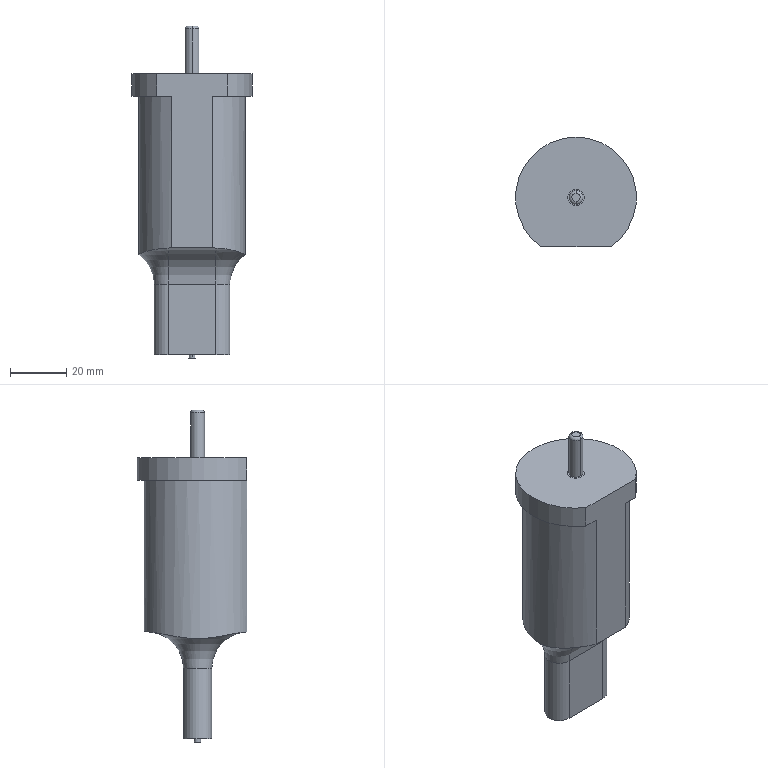Part | STEP file | 1_id290_x_t | 1 solid | 28 faces | box 43 x 39 x 118.2 mm | volume 84183 mm3 | cylinder 14 | plane 10 | torus 4 | commonest cylinder face diameters 2.26 x2 5 x2 6 x2 10.07 x2 26 x2 38 x2
STEP:
#1=CARTESIAN_POINT('',(3411.,-73.993,30.458));
#2=VERTEX_POINT('',#1);
#3=CARTESIAN_POINT('',(3412.101,-74.5,30.489));
#4=VERTEX_POINT('',#3);
#5=CARTESIAN_POINT('',(3411.,-73.993,30.458));
#6=CARTESIAN_POINT('',(3411.361,-74.173,30.473));
#7=CARTESIAN_POINT('',(3411.729,-74.343,30.483));
#8=CARTESIAN_POINT('',(3412.101,-74.5,30.489));
#9=B_SPLINE_CURVE_WITH_KNOTS('',3,(#5,#6,#7,#8),.UNSPECIFIED.,.F.,.F.,(4,4),(0.,1.),.UNSPECIFIED.);
#10=EDGE_CURVE('',#2,#4,#9,.T.);
#11=ORIENTED_EDGE('',*,*,#10,.T.);
#12=CARTESIAN_POINT('',(3412.101,-74.5,84.5));
#13=VERTEX_POINT('',#12);
#14=CARTESIAN_POINT('',(3412.101,-74.5,38.5));
#15=DIRECTION('',(0.,0.,1.));
#16=VECTOR('',#15,1.);
#17=LINE('',#14,#16);
#18=EDGE_CURVE('',#4,#13,#17,.T.);
#19=ORIENTED_EDGE('',*,*,#18,.T.);
#20=CARTESIAN_POINT('',(3419.5,-38.,84.5));
#21=VERTEX_POINT('',#20);
#22=CARTESIAN_POINT('',(3419.5,-57.,84.5));
#23=DIRECTION('',(0.,0.,1.));
#24=DIRECTION('',(0.,1.,0.));
#25=AXIS2_PLACEMENT_3D('',#22,#23,#24);
#26=CIRCLE('',#25,19.);
#27=EDGE_CURVE('',#21,#13,#26,.T.);
#28=ORIENTED_EDGE('',*,*,#27,.F.);
#29=CARTESIAN_POINT('',(3419.5,-38.,30.5));
#30=VERTEX_POINT('',#29);
#31=CARTESIAN_POINT('',(3419.5,-38.,38.5));
#32=DIRECTION('',(0.,0.,1.));
#33=VECTOR('',#32,1.);
#34=LINE('',#31,#33);
#35=EDGE_CURVE('',#30,#21,#34,.T.);
#36=ORIENTED_EDGE('',*,*,#35,.F.);
#37=CARTESIAN_POINT('',(3413.522,-38.965,30.5));
#38=VERTEX_POINT('',#37);
#39=CARTESIAN_POINT('',(3419.5,-57.,30.5));
#40=DIRECTION('',(0.,0.,1.));
#41=DIRECTION('',(0.,1.,0.));
#42=AXIS2_PLACEMENT_3D('',#39,#40,#41);
#43=CIRCLE('',#42,19.);
#44=EDGE_CURVE('',#30,#38,#43,.T.);
#45=ORIENTED_EDGE('',*,*,#44,.T.);
#46=CARTESIAN_POINT('',(3411.,-40.007,30.458));
#47=VERTEX_POINT('',#46);
#48=CARTESIAN_POINT('',(3413.522,-38.965,30.5));
#49=CARTESIAN_POINT('',(3412.658,-39.251,30.5));
#50=CARTESIAN_POINT('',(3411.813,-39.601,30.491));
#51=CARTESIAN_POINT('',(3411.,-40.007,30.458));
#52=B_SPLINE_CURVE_WITH_KNOTS('',3,(#48,#49,#50,#51),.UNSPECIFIED.,.F.,.F.,(4,4),(0.,1.),.UNSPECIFIED.);
#53=EDGE_CURVE('',#38,#47,#52,.T.);
#54=ORIENTED_EDGE('',*,*,#53,.T.);
#55=CARTESIAN_POINT('',(3411.,-40.007,30.458));
#56=CARTESIAN_POINT('',(3407.815,-41.601,30.33));
#57=CARTESIAN_POINT('',(3405.165,-44.053,29.874));
#58=CARTESIAN_POINT('',(3401.509,-49.97,28.735));
#59=CARTESIAN_POINT('',(3400.502,-53.482,28.095));
#60=CARTESIAN_POINT('',(3400.498,-60.5,28.093));
#61=CARTESIAN_POINT('',(3401.497,-64.005,28.73));
#62=CARTESIAN_POINT('',(3405.163,-69.948,29.874));
#63=CARTESIAN_POINT('',(3407.814,-72.399,30.33));
#64=CARTESIAN_POINT('',(3411.,-73.993,30.458));
#65=B_SPLINE_CURVE_WITH_KNOTS('',3,(#55,#56,#57,#58,#59,#60,#61,#62,#63,#64),.UNSPECIFIED.,.F.,.F.,(4,2,2,2,4),(0.,0.25,0.5,0.75,1.),.UNSPECIFIED.);
#66=EDGE_CURVE('',#47,#2,#65,.T.);
#67=ORIENTED_EDGE('',*,*,#66,.T.);
#68=EDGE_LOOP('',(#11,#19,#28,#36,#45,#54,#67));
#69=FACE_OUTER_BOUND('',#68,.T.);
#70=CARTESIAN_POINT('',(3419.5,-57.,38.5));
#71=DIRECTION('',(0.,0.,-1.));
#72=DIRECTION('',(0.,-1.,0.));
#73=AXIS2_PLACEMENT_3D('',#70,#71,#72);
#74=CYLINDRICAL_SURFACE('',#73,19.);
#75=ADVANCED_FACE('',(#69),#74,.T.);
#76=CARTESIAN_POINT('',(3419.5,-35.5,84.5));
#77=VERTEX_POINT('',#76);
#78=CARTESIAN_POINT('',(3407.01,-74.5,84.5));
#79=VERTEX_POINT('',#78);
#80=CARTESIAN_POINT('',(3419.5,-57.,84.5));
#81=DIRECTION('',(0.,0.,1.));
#82=DIRECTION('',(0.,1.,0.));
#83=AXIS2_PLACEMENT_3D('',#80,#81,#82);
#84=CIRCLE('',#83,21.5);
#85=EDGE_CURVE('',#77,#79,#84,.T.);
#86=ORIENTED_EDGE('',*,*,#85,.T.);
#87=CARTESIAN_POINT('',(3407.01,-74.5,92.5));
#88=VERTEX_POINT('',#87);
#89=CARTESIAN_POINT('',(3407.01,-74.5,88.5));
#90=DIRECTION('',(0.,0.,-1.));
#91=VECTOR('',#90,1.);
#92=LINE('',#89,#91);
#93=EDGE_CURVE('',#88,#79,#92,.T.);
#94=ORIENTED_EDGE('',*,*,#93,.F.);
#95=CARTESIAN_POINT('',(3419.5,-35.5,92.5));
#96=VERTEX_POINT('',#95);
#97=CARTESIAN_POINT('',(3419.5,-57.,92.5));
#98=DIRECTION('',(0.,0.,1.));
#99=DIRECTION('',(0.,1.,0.));
#100=AXIS2_PLACEMENT_3D('',#97,#98,#99);
#101=CIRCLE('',#100,21.5);
#102=EDGE_CURVE('',#96,#88,#101,.T.);
#103=ORIENTED_EDGE('',*,*,#102,.F.);
#104=CARTESIAN_POINT('',(3419.5,-35.5,88.5));
#105=DIRECTION('',(0.,0.,1.));
#106=VECTOR('',#105,1.);
#107=LINE('',#104,#106);
#108=EDGE_CURVE('',#77,#96,#107,.T.);
#109=ORIENTED_EDGE('',*,*,#108,.F.);
#110=EDGE_LOOP('',(#86,#94,#103,#109));
#111=FACE_OUTER_BOUND('',#110,.T.);
#112=CARTESIAN_POINT('',(3419.5,-57.,88.5));
#113=DIRECTION('',(0.,0.,-1.));
#114=DIRECTION('',(0.,-1.,0.));
#115=AXIS2_PLACEMENT_3D('',#112,#113,#114);
#116=CYLINDRICAL_SURFACE('',#115,21.5);
#117=ADVANCED_FACE('',(#111),#116,.T.);
#118=CARTESIAN_POINT('',(3431.99,-74.5,92.5));
#119=VERTEX_POINT('',#118);
#120=CARTESIAN_POINT('',(3419.5,-57.,92.5));
#121=DIRECTION('',(0.,0.,1.));
#122=DIRECTION('',(0.,1.,0.));
#123=AXIS2_PLACEMENT_3D('',#120,#121,#122);
#124=CIRCLE('',#123,21.5);
#125=EDGE_CURVE('',#119,#96,#124,.T.);
#126=ORIENTED_EDGE('',*,*,#125,.F.);
#127=CARTESIAN_POINT('',(3431.99,-74.5,84.5));
#128=VERTEX_POINT('',#127);
#129=CARTESIAN_POINT('',(3431.99,-74.5,88.5));
#130=DIRECTION('',(0.,0.,-1.));
#131=VECTOR('',#130,1.);
#132=LINE('',#129,#131);
#133=EDGE_CURVE('',#119,#128,#132,.T.);
#134=ORIENTED_EDGE('',*,*,#133,.T.);
#135=CARTESIAN_POINT('',(3419.5,-57.,84.5));
#136=DIRECTION('',(0.,0.,1.));
#137=DIRECTION('',(0.,1.,0.));
#138=AXIS2_PLACEMENT_3D('',#135,#136,#137);
#139=CIRCLE('',#138,21.5);
#140=EDGE_CURVE('',#128,#77,#139,.T.);
#141=ORIENTED_EDGE('',*,*,#140,.T.);
#142=ORIENTED_EDGE('',*,*,#108,.T.);
#143=EDGE_LOOP('',(#126,#134,#141,#142));
#144=FACE_OUTER_BOUND('',#143,.T.);
#145=CARTESIAN_POINT('',(3419.5,-57.,88.5));
#146=DIRECTION('',(0.,0.,-1.));
#147=DIRECTION('',(0.,-1.,0.));
#148=AXIS2_PLACEMENT_3D('',#145,#146,#147);
#149=CYLINDRICAL_SURFACE('',#148,21.5);
#150=ADVANCED_FACE('',(#144),#149,.T.);
#151=ORIENTED_EDGE('',*,*,#140,.F.);
#152=CARTESIAN_POINT('',(3426.899,-74.5,84.5));
#153=VERTEX_POINT('',#152);
#154=CARTESIAN_POINT('',(3419.5,-74.5,84.5));
#155=DIRECTION('',(-1.,0.,0.));
#156=VECTOR('',#155,1.);
#157=LINE('',#154,#156);
#158=EDGE_CURVE('',#128,#153,#157,.T.);
#159=ORIENTED_EDGE('',*,*,#158,.T.);
#160=CARTESIAN_POINT('',(3419.5,-57.,84.5));
#161=DIRECTION('',(0.,0.,1.));
#162=DIRECTION('',(0.,1.,0.));
#163=AXIS2_PLACEMENT_3D('',#160,#161,#162);
#164=CIRCLE('',#163,19.);
#165=EDGE_CURVE('',#153,#21,#164,.T.);
#166=ORIENTED_EDGE('',*,*,#165,.T.);
#167=ORIENTED_EDGE('',*,*,#27,.T.);
#168=CARTESIAN_POINT('',(3419.5,-74.5,84.5));
#169=DIRECTION('',(-1.,0.,0.));
#170=VECTOR('',#169,1.);
#171=LINE('',#168,#170);
#172=EDGE_CURVE('',#13,#79,#171,.T.);
#173=ORIENTED_EDGE('',*,*,#172,.T.);
#174=ORIENTED_EDGE('',*,*,#85,.F.);
#175=EDGE_LOOP('',(#151,#159,#166,#167,#173,#174));
#176=FACE_OUTER_BOUND('',#175,.T.);
#177=CARTESIAN_POINT('',(3419.5,-36.75,84.5));
#178=DIRECTION('',(0.,0.,-1.));
#179=DIRECTION('',(0.,1.,0.));
#180=AXIS2_PLACEMENT_3D('',#177,#178,#179);
#181=PLANE('',#180);
#182=ADVANCED_FACE('',(#176),#181,.T.);
#183=CARTESIAN_POINT('',(3426.899,-74.5,30.489));
#184=VERTEX_POINT('',#183);
#185=CARTESIAN_POINT('',(3457.5,-74.5,30.489));
#186=DIRECTION('',(1.,0.,0.));
#187=VECTOR('',#186,1.);
#188=LINE('',#185,#187);
#189=EDGE_CURVE('',#4,#184,#188,.T.);
#190=ORIENTED_EDGE('',*,*,#189,.F.);
#191=ORIENTED_EDGE('',*,*,#10,.F.);
#192=CARTESIAN_POINT('',(3411.,-62.035,17.5));
#193=VERTEX_POINT('',#192);
#194=CARTESIAN_POINT('',(3411.,-75.035,17.5));
#195=DIRECTION('',(-1.,0.,0.));
#196=DIRECTION('',(0.,-1.,0.));
#197=AXIS2_PLACEMENT_3D('',#194,#195,#196);
#198=CIRCLE('',#197,13.);
#199=EDGE_CURVE('',#2,#193,#198,.T.);
#200=ORIENTED_EDGE('',*,*,#199,.T.);
#201=CARTESIAN_POINT('',(3428.,-62.035,17.5));
#202=VERTEX_POINT('',#201);
#203=CARTESIAN_POINT('',(3457.5,-62.035,17.5));
#204=DIRECTION('',(-1.,0.,0.));
#205=VECTOR('',#204,1.);
#206=LINE('',#203,#205);
#207=EDGE_CURVE('',#202,#193,#206,.T.);
#208=ORIENTED_EDGE('',*,*,#207,.F.);
#209=CARTESIAN_POINT('',(3428.,-73.993,30.458));
#210=VERTEX_POINT('',#209);
#211=CARTESIAN_POINT('',(3428.,-75.035,17.5));
#212=DIRECTION('',(1.,0.,0.));
#213=DIRECTION('',(0.,-1.,0.));
#214=AXIS2_PLACEMENT_3D('',#211,#212,#213);
#215=CIRCLE('',#214,13.);
#216=EDGE_CURVE('',#202,#210,#215,.T.);
#217=ORIENTED_EDGE('',*,*,#216,.T.);
#218=CARTESIAN_POINT('',(3426.899,-74.5,30.489));
#219=CARTESIAN_POINT('',(3427.272,-74.343,30.483));
#220=CARTESIAN_POINT('',(3427.639,-74.173,30.473));
#221=CARTESIAN_POINT('',(3428.,-73.993,30.458));
#222=B_SPLINE_CURVE_WITH_KNOTS('',3,(#218,#219,#220,#221),.UNSPECIFIED.,.F.,.F.,(4,4),(0.,1.),.UNSPECIFIED.);
#223=EDGE_CURVE('',#184,#210,#222,.T.);
#224=ORIENTED_EDGE('',*,*,#223,.F.);
#225=EDGE_LOOP('',(#190,#191,#200,#208,#217,#224));
#226=FACE_OUTER_BOUND('',#225,.T.);
#227=CARTESIAN_POINT('',(3457.5,-75.035,17.5));
#228=DIRECTION('',(1.,0.,0.));
#229=DIRECTION('',(0.,-1.,0.));
#230=AXIS2_PLACEMENT_3D('',#227,#228,#229);
#231=CYLINDRICAL_SURFACE('',#230,13.);
#232=ADVANCED_FACE('',(#226),#231,.F.);
#233=ORIENTED_EDGE('',*,*,#165,.F.);
#234=CARTESIAN_POINT('',(3426.899,-74.5,38.5));
#235=DIRECTION('',(0.,0.,-1.));
#236=VECTOR('',#235,1.);
#237=LINE('',#234,#236);
#238=EDGE_CURVE('',#153,#184,#237,.T.);
#239=ORIENTED_EDGE('',*,*,#238,.T.);
#240=ORIENTED_EDGE('',*,*,#223,.T.);
#241=CARTESIAN_POINT('',(3428.,-40.007,30.458));
#242=VERTEX_POINT('',#241);
#243=CARTESIAN_POINT('',(3428.,-73.993,30.458));
#244=CARTESIAN_POINT('',(3431.185,-72.399,30.33));
#245=CARTESIAN_POINT('',(3433.835,-69.947,29.874));
#246=CARTESIAN_POINT('',(3437.491,-64.03,28.735));
#247=CARTESIAN_POINT('',(3438.498,-60.518,28.095));
#248=CARTESIAN_POINT('',(3438.502,-53.5,28.093));
#249=CARTESIAN_POINT('',(3437.503,-49.995,28.73));
#250=CARTESIAN_POINT('',(3433.837,-44.052,29.874));
#251=CARTESIAN_POINT('',(3431.186,-41.601,30.33));
#252=CARTESIAN_POINT('',(3428.,-40.007,30.458));
#253=B_SPLINE_CURVE_WITH_KNOTS('',3,(#243,#244,#245,#246,#247,#248,#249,#250,#251,#252),.UNSPECIFIED.,.F.,.F.,(4,2,2,2,4),(0.,0.25,0.5,0.75,1.),.UNSPECIFIED.);
#254=EDGE_CURVE('',#210,#242,#253,.T.);
#255=ORIENTED_EDGE('',*,*,#254,.T.);
#256=CARTESIAN_POINT('',(3425.478,-38.965,30.5));
#257=VERTEX_POINT('',#256);
#258=CARTESIAN_POINT('',(3428.,-40.007,30.458));
#259=CARTESIAN_POINT('',(3427.187,-39.601,30.491));
#260=CARTESIAN_POINT('',(3426.342,-39.251,30.5));
#261=CARTESIAN_POINT('',(3425.478,-38.965,30.5));
#262=B_SPLINE_CURVE_WITH_KNOTS('',3,(#258,#259,#260,#261),.UNSPECIFIED.,.F.,.F.,(4,4),(0.,1.),.UNSPECIFIED.);
#263=EDGE_CURVE('',#242,#257,#262,.T.);
#264=ORIENTED_EDGE('',*,*,#263,.T.);
#265=CARTESIAN_POINT('',(3419.5,-57.,30.5));
#266=DIRECTION('',(0.,0.,1.));
#267=DIRECTION('',(0.,1.,0.));
#268=AXIS2_PLACEMENT_3D('',#265,#266,#267);
#269=CIRCLE('',#268,19.);
#270=EDGE_CURVE('',#257,#30,#269,.T.);
#271=ORIENTED_EDGE('',*,*,#270,.T.);
#272=ORIENTED_EDGE('',*,*,#35,.T.);
#273=EDGE_LOOP('',(#233,#239,#240,#255,#264,#271,#272));
#274=FACE_OUTER_BOUND('',#273,.T.);
#275=CARTESIAN_POINT('',(3419.5,-57.,38.5));
#276=DIRECTION('',(0.,0.,-1.));
#277=DIRECTION('',(0.,-1.,0.));
#278=AXIS2_PLACEMENT_3D('',#275,#276,#277);
#279=CYLINDRICAL_SURFACE('',#278,19.);
#280=ADVANCED_FACE('',(#274),#279,.T.);
#281=CARTESIAN_POINT('',(3419.5,-54.,92.5));
#282=VERTEX_POINT('',#281);
#283=CARTESIAN_POINT('',(3419.5,-60.,92.5));
#284=VERTEX_POINT('',#283);
#285=CARTESIAN_POINT('',(3419.5,-57.,92.5));
#286=DIRECTION('',(0.,0.,-1.));
#287=DIRECTION('',(0.,-1.,0.));
#288=AXIS2_PLACEMENT_3D('',#285,#286,#287);
#289=CIRCLE('',#288,3.);
#290=EDGE_CURVE('',#282,#284,#289,.T.);
#291=ORIENTED_EDGE('',*,*,#290,.T.);
#292=CARTESIAN_POINT('',(3419.5,-57.,92.5));
#293=DIRECTION('',(0.,0.,-1.));
#294=DIRECTION('',(0.,-1.,0.));
#295=AXIS2_PLACEMENT_3D('',#292,#293,#294);
#296=CIRCLE('',#295,3.);
#297=EDGE_CURVE('',#284,#282,#296,.T.);
#298=ORIENTED_EDGE('',*,*,#297,.T.);
#299=EDGE_LOOP('',(#291,#298));
#300=FACE_BOUND('',#299,.T.);
#301=ORIENTED_EDGE('',*,*,#102,.T.);
#302=CARTESIAN_POINT('',(3419.5,-74.5,92.5));
#303=DIRECTION('',(-1.,0.,0.));
#304=VECTOR('',#303,1.);
#305=LINE('',#302,#304);
#306=EDGE_CURVE('',#119,#88,#305,.T.);
#307=ORIENTED_EDGE('',*,*,#306,.F.);
#308=ORIENTED_EDGE('',*,*,#125,.T.);
#309=EDGE_LOOP('',(#301,#307,#308));
#310=FACE_BOUND('',#309,.T.);
#311=CARTESIAN_POINT('',(3419.5,-46.25,92.5));
#312=DIRECTION('',(0.,0.,1.));
#313=DIRECTION('',(0.,-1.,0.));
#314=AXIS2_PLACEMENT_3D('',#311,#312,#313);
#315=PLANE('',#314);
#316=ADVANCED_FACE('',(#300,#310),#315,.T.);
#317=CARTESIAN_POINT('',(3419.5,-58.13,-7.5));
#318=VERTEX_POINT('',#317);
#319=CARTESIAN_POINT('',(3419.5,-58.13,-8.7));
#320=VERTEX_POINT('',#319);
#321=CARTESIAN_POINT('',(3419.5,-58.13,-7.5));
#322=DIRECTION('',(0.,0.,-1.));
#323=VECTOR('',#322,1.);
#324=LINE('',#321,#323);
#325=EDGE_CURVE('',#318,#320,#324,.T.);
#326=ORIENTED_EDGE('',*,*,#325,.F.);
#327=CARTESIAN_POINT('',(3419.5,-55.87,-7.5));
#328=VERTEX_POINT('',#327);
#329=CARTESIAN_POINT('',(3419.5,-57.,-7.5));
#330=DIRECTION('',(0.,0.,1.));
#331=DIRECTION('',(0.,-1.,0.));
#332=AXIS2_PLACEMENT_3D('',#329,#330,#331);
#333=CIRCLE('',#332,1.13);
#334=EDGE_CURVE('',#328,#318,#333,.T.);
#335=ORIENTED_EDGE('',*,*,#334,.F.);
#336=CARTESIAN_POINT('',(3419.5,-55.87,-8.7));
#337=VERTEX_POINT('',#336);
#338=CARTESIAN_POINT('',(3419.5,-55.87,-7.5));
#339=DIRECTION('',(0.,0.,1.));
#340=VECTOR('',#339,1.);
#341=LINE('',#338,#340);
#342=EDGE_CURVE('',#337,#328,#341,.T.);
#343=ORIENTED_EDGE('',*,*,#342,.F.);
#344=CARTESIAN_POINT('',(3419.5,-57.,-8.7));
#345=DIRECTION('',(0.,0.,1.));
#346=DIRECTION('',(0.,-1.,0.));
#347=AXIS2_PLACEMENT_3D('',#344,#345,#346);
#348=CIRCLE('',#347,1.13);
#349=EDGE_CURVE('',#337,#320,#348,.T.);
#350=ORIENTED_EDGE('',*,*,#349,.T.);
#351=EDGE_LOOP('',(#326,#335,#343,#350));
#352=FACE_OUTER_BOUND('',#351,.T.);
#353=CARTESIAN_POINT('',(3419.5,-57.,-7.5));
#354=DIRECTION('',(0.,0.,1.));
#355=DIRECTION('',(0.,1.,0.));
#356=AXIS2_PLACEMENT_3D('',#353,#354,#355);
#357=CYLINDRICAL_SURFACE('',#356,1.13);
#358=ADVANCED_FACE('',(#352),#357,.T.);
#359=CARTESIAN_POINT('',(3419.5,-59.5,108.5));
#360=VERTEX_POINT('',#359);
#361=CARTESIAN_POINT('',(3419.5,-59.5,92.6));
#362=VERTEX_POINT('',#361);
#363=CARTESIAN_POINT('',(3419.5,-59.5,100.55));
#364=DIRECTION('',(0.,0.,-1.));
#365=VECTOR('',#364,1.);
#366=LINE('',#363,#365);
#367=EDGE_CURVE('',#360,#362,#366,.T.);
#368=ORIENTED_EDGE('',*,*,#367,.F.);
#369=CARTESIAN_POINT('',(3419.5,-54.5,108.5));
#370=VERTEX_POINT('',#369);
#371=CARTESIAN_POINT('',(3419.5,-57.,108.5));
#372=DIRECTION('',(0.,0.,-1.));
#373=DIRECTION('',(0.,-1.,0.));
#374=AXIS2_PLACEMENT_3D('',#371,#372,#373);
#375=CIRCLE('',#374,2.5);
#376=EDGE_CURVE('',#360,#370,#375,.T.);
#377=ORIENTED_EDGE('',*,*,#376,.T.);
#378=CARTESIAN_POINT('',(3419.5,-54.5,92.6));
#379=VERTEX_POINT('',#378);
#380=CARTESIAN_POINT('',(3419.5,-54.5,100.55));
#381=DIRECTION('',(0.,0.,1.));
#382=VECTOR('',#381,1.);
#383=LINE('',#380,#382);
#384=EDGE_CURVE('',#379,#370,#383,.T.);
#385=ORIENTED_EDGE('',*,*,#384,.F.);
#386=CARTESIAN_POINT('',(3419.5,-57.,92.6));
#387=DIRECTION('',(0.,0.,-1.));
#388=DIRECTION('',(0.,-1.,0.));
#389=AXIS2_PLACEMENT_3D('',#386,#387,#388);
#390=CIRCLE('',#389,2.5);
#391=EDGE_CURVE('',#362,#379,#390,.T.);
#392=ORIENTED_EDGE('',*,*,#391,.F.);
#393=EDGE_LOOP('',(#368,#377,#385,#392));
#394=FACE_OUTER_BOUND('',#393,.T.);
#395=CARTESIAN_POINT('',(3419.5,-57.,100.55));
#396=DIRECTION('',(0.,0.,1.));
#397=DIRECTION('',(0.,1.,0.));
#398=AXIS2_PLACEMENT_3D('',#395,#396,#397);
#399=CYLINDRICAL_SURFACE('',#398,2.5);
#400=ADVANCED_FACE('',(#394),#399,.T.);
#401=CARTESIAN_POINT('',(3419.5,-55.5,109.5));
#402=VERTEX_POINT('',#401);
#403=CARTESIAN_POINT('',(3419.5,-55.5,108.5));
#404=DIRECTION('',(-1.,0.,0.));
#405=DIRECTION('',(0.,1.,0.));
#406=AXIS2_PLACEMENT_3D('',#403,#404,#405);
#407=CIRCLE('',#406,1.);
#408=EDGE_CURVE('',#402,#370,#407,.T.);
#409=ORIENTED_EDGE('',*,*,#408,.F.);
#410=CARTESIAN_POINT('',(3419.5,-58.5,109.5));
#411=VERTEX_POINT('',#410);
#412=CARTESIAN_POINT('',(3419.5,-57.,109.5));
#413=DIRECTION('',(0.,0.,-1.));
#414=DIRECTION('',(0.,-1.,0.));
#415=AXIS2_PLACEMENT_3D('',#412,#413,#414);
#416=CIRCLE('',#415,1.5);
#417=EDGE_CURVE('',#402,#411,#416,.T.);
#418=ORIENTED_EDGE('',*,*,#417,.T.);
#419=CARTESIAN_POINT('',(3419.5,-58.5,108.5));
#420=DIRECTION('',(-1.,0.,0.));
#421=DIRECTION('',(0.,-1.,0.));
#422=AXIS2_PLACEMENT_3D('',#419,#420,#421);
#423=CIRCLE('',#422,1.);
#424=EDGE_CURVE('',#360,#411,#423,.T.);
#425=ORIENTED_EDGE('',*,*,#424,.F.);
#426=CARTESIAN_POINT('',(3419.5,-57.,108.5));
#427=DIRECTION('',(0.,0.,-1.));
#428=DIRECTION('',(0.,-1.,0.));
#429=AXIS2_PLACEMENT_3D('',#426,#427,#428);
#430=CIRCLE('',#429,2.5);
#431=EDGE_CURVE('',#370,#360,#430,.T.);
#432=ORIENTED_EDGE('',*,*,#431,.F.);
#433=EDGE_LOOP('',(#409,#418,#425,#432));
#434=FACE_OUTER_BOUND('',#433,.T.);
#435=CARTESIAN_POINT('',(3419.5,-57.,108.5));
#436=DIRECTION('',(0.,0.,-1.));
#437=DIRECTION('',(0.,-1.,0.));
#438=AXIS2_PLACEMENT_3D('',#435,#436,#437);
#439=TOROIDAL_SURFACE('',#438,1.5,1.);
#440=ADVANCED_FACE('',(#434),#439,.T.);
#441=CARTESIAN_POINT('',(3419.5,-60.,92.6));
#442=VERTEX_POINT('',#441);
#443=CARTESIAN_POINT('',(3419.5,-60.,92.55));
#444=DIRECTION('',(0.,0.,-1.));
#445=VECTOR('',#444,1.);
#446=LINE('',#443,#445);
#447=EDGE_CURVE('',#442,#284,#446,.T.);
#448=ORIENTED_EDGE('',*,*,#447,.F.);
#449=CARTESIAN_POINT('',(3419.5,-54.,92.6));
#450=VERTEX_POINT('',#449);
#451=CARTESIAN_POINT('',(3419.5,-57.,92.6));
#452=DIRECTION('',(0.,0.,-1.));
#453=DIRECTION('',(0.,-1.,0.));
#454=AXIS2_PLACEMENT_3D('',#451,#452,#453);
#455=CIRCLE('',#454,3.);
#456=EDGE_CURVE('',#442,#450,#455,.T.);
#457=ORIENTED_EDGE('',*,*,#456,.T.);
#458=CARTESIAN_POINT('',(3419.5,-54.,92.55));
#459=DIRECTION('',(0.,0.,1.));
#460=VECTOR('',#459,1.);
#461=LINE('',#458,#460);
#462=EDGE_CURVE('',#282,#450,#461,.T.);
#463=ORIENTED_EDGE('',*,*,#462,.F.);
#464=ORIENTED_EDGE('',*,*,#297,.F.);
#465=EDGE_LOOP('',(#448,#457,#463,#464));
#466=FACE_OUTER_BOUND('',#465,.T.);
#467=CARTESIAN_POINT('',(3419.5,-57.,87.05));
#468=DIRECTION('',(0.,0.,1.));
#469=DIRECTION('',(0.,1.,0.));
#470=AXIS2_PLACEMENT_3D('',#467,#468,#469);
#471=CYLINDRICAL_SURFACE('',#470,3.);
#472=ADVANCED_FACE('',(#466),#471,.T.);
#473=ORIENTED_EDGE('',*,*,#447,.T.);
#474=ORIENTED_EDGE('',*,*,#290,.F.);
#475=ORIENTED_EDGE('',*,*,#462,.T.);
#476=CARTESIAN_POINT('',(3419.5,-57.,92.6));
#477=DIRECTION('',(0.,0.,-1.));
#478=DIRECTION('',(0.,-1.,0.));
#479=AXIS2_PLACEMENT_3D('',#476,#477,#478);
#480=CIRCLE('',#479,3.);
#481=EDGE_CURVE('',#450,#442,#480,.T.);
#482=ORIENTED_EDGE('',*,*,#481,.T.);
#483=EDGE_LOOP('',(#473,#474,#475,#482));
#484=FACE_OUTER_BOUND('',#483,.T.);
#485=CARTESIAN_POINT('',(3419.5,-57.,87.05));
#486=DIRECTION('',(0.,0.,1.));
#487=DIRECTION('',(0.,1.,0.));
#488=AXIS2_PLACEMENT_3D('',#485,#486,#487);
#489=CYLINDRICAL_SURFACE('',#488,3.);
#490=ADVANCED_FACE('',(#484),#489,.T.);
#491=CARTESIAN_POINT('',(3419.5,-57.,109.5));
#492=DIRECTION('',(0.,0.,-1.));
#493=DIRECTION('',(0.,-1.,0.));
#494=AXIS2_PLACEMENT_3D('',#491,#492,#493);
#495=CIRCLE('',#494,1.5);
#496=EDGE_CURVE('',#411,#402,#495,.T.);
#497=ORIENTED_EDGE('',*,*,#496,.F.);
#498=ORIENTED_EDGE('',*,*,#417,.F.);
#499=EDGE_LOOP('',(#497,#498));
#500=FACE_OUTER_BOUND('',#499,.T.);
#501=CARTESIAN_POINT('',(3419.5,-57.75,109.5));
#502=DIRECTION('',(0.,0.,1.));
#503=DIRECTION('',(0.,-1.,0.));
#504=AXIS2_PLACEMENT_3D('',#501,#502,#503);
#505=PLANE('',#504);
#506=ADVANCED_FACE('',(#500),#505,.T.);
#507=ORIENTED_EDGE('',*,*,#408,.T.);
#508=ORIENTED_EDGE('',*,*,#376,.F.);
#509=ORIENTED_EDGE('',*,*,#424,.T.);
#510=ORIENTED_EDGE('',*,*,#496,.T.);
#511=EDGE_LOOP('',(#507,#508,#509,#510));
#512=FACE_OUTER_BOUND('',#511,.T.);
#513=CARTESIAN_POINT('',(3419.5,-57.,108.5));
#514=DIRECTION('',(0.,0.,-1.));
#515=DIRECTION('',(0.,-1.,0.));
#516=AXIS2_PLACEMENT_3D('',#513,#514,#515);
#517=TOROIDAL_SURFACE('',#516,1.5,1.);
#518=ADVANCED_FACE('',(#512),#517,.T.);
#519=ORIENTED_EDGE('',*,*,#367,.T.);
#520=CARTESIAN_POINT('',(3419.5,-57.,92.6));
#521=DIRECTION('',(0.,0.,-1.));
#522=DIRECTION('',(0.,-1.,0.));
#523=AXIS2_PLACEMENT_3D('',#520,#521,#522);
#524=CIRCLE('',#523,2.5);
#525=EDGE_CURVE('',#379,#362,#524,.T.);
#526=ORIENTED_EDGE('',*,*,#525,.F.);
#527=ORIENTED_EDGE('',*,*,#384,.T.);
#528=ORIENTED_EDGE('',*,*,#431,.T.);
#529=EDGE_LOOP('',(#519,#526,#527,#528));
#530=FACE_OUTER_BOUND('',#529,.T.);
#531=CARTESIAN_POINT('',(3419.5,-57.,100.55));
#532=DIRECTION('',(0.,0.,1.));
#533=DIRECTION('',(0.,1.,0.));
#534=AXIS2_PLACEMENT_3D('',#531,#532,#533);
#535=CYLINDRICAL_SURFACE('',#534,2.5);
#536=ADVANCED_FACE('',(#530),#535,.T.);
#537=ORIENTED_EDGE('',*,*,#456,.F.);
#538=ORIENTED_EDGE('',*,*,#481,.F.);
#539=EDGE_LOOP('',(#537,#538));
#540=FACE_BOUND('',#539,.T.);
#541=ORIENTED_EDGE('',*,*,#391,.T.);
#542=ORIENTED_EDGE('',*,*,#525,.T.);
#543=EDGE_LOOP('',(#541,#542));
#544=FACE_BOUND('',#543,.T.);
#545=CARTESIAN_POINT('',(3419.5,-59.75,92.6));
#546=DIRECTION('',(0.,0.,1.));
#547=DIRECTION('',(0.,-1.,0.));
#548=AXIS2_PLACEMENT_3D('',#545,#546,#547);
#549=PLANE('',#548);
#550=ADVANCED_FACE('',(#540,#544),#549,.T.);
#551=ORIENTED_EDGE('',*,*,#325,.T.);
#552=CARTESIAN_POINT('',(3419.5,-57.,-8.7));
#553=DIRECTION('',(0.,0.,1.));
#554=DIRECTION('',(0.,-1.,0.));
#555=AXIS2_PLACEMENT_3D('',#552,#553,#554);
#556=CIRCLE('',#555,1.13);
#557=EDGE_CURVE('',#320,#337,#556,.T.);
#558=ORIENTED_EDGE('',*,*,#557,.T.);
#559=ORIENTED_EDGE('',*,*,#342,.T.);
#560=CARTESIAN_POINT('',(3419.5,-57.,-7.5));
#561=DIRECTION('',(0.,0.,1.));
#562=DIRECTION('',(0.,-1.,0.));
#563=AXIS2_PLACEMENT_3D('',#560,#561,#562);
#564=CIRCLE('',#563,1.13);
#565=EDGE_CURVE('',#318,#328,#564,.T.);
#566=ORIENTED_EDGE('',*,*,#565,.F.);
#567=EDGE_LOOP('',(#551,#558,#559,#566));
#568=FACE_OUTER_BOUND('',#567,.T.);
#569=CARTESIAN_POINT('',(3419.5,-57.,-7.5));
#570=DIRECTION('',(0.,0.,1.));
#571=DIRECTION('',(0.,1.,0.));
#572=AXIS2_PLACEMENT_3D('',#569,#570,#571);
#573=CYLINDRICAL_SURFACE('',#572,1.13);
#574=ADVANCED_FACE('',(#568),#573,.T.);
#575=ORIENTED_EDGE('',*,*,#557,.F.);
#576=ORIENTED_EDGE('',*,*,#349,.F.);
#577=EDGE_LOOP('',(#575,#576));
#578=FACE_OUTER_BOUND('',#577,.T.);
#579=CARTESIAN_POINT('',(3419.5,-57.,-8.7));
#580=DIRECTION('',(0.,0.,1.));
#581=DIRECTION('',(0.,1.,0.));
#582=AXIS2_PLACEMENT_3D('',#579,#580,#581);
#583=PLANE('',#582);
#584=ADVANCED_FACE('',(#578),#583,.F.);
#585=CARTESIAN_POINT('',(3411.,-62.035,-7.5));
#586=VERTEX_POINT('',#585);
#587=CARTESIAN_POINT('',(3411.,-51.965,-7.5));
#588=VERTEX_POINT('',#587);
#589=CARTESIAN_POINT('',(3411.,-57.,-7.5));
#590=DIRECTION('',(0.,0.,-1.));
#591=DIRECTION('',(0.,-1.,0.));
#592=AXIS2_PLACEMENT_3D('',#589,#590,#591);
#593=CIRCLE('',#592,5.035);
#594=EDGE_CURVE('',#586,#588,#593,.T.);
#595=ORIENTED_EDGE('',*,*,#594,.F.);
#596=CARTESIAN_POINT('',(3411.,-62.035,5.));
#597=DIRECTION('',(0.,0.,1.));
#598=VECTOR('',#597,1.);
#599=LINE('',#596,#598);
#600=EDGE_CURVE('',#586,#193,#599,.T.);
#601=ORIENTED_EDGE('',*,*,#600,.T.);
#602=CARTESIAN_POINT('',(3411.,-51.965,17.5));
#603=VERTEX_POINT('',#602);
#604=CARTESIAN_POINT('',(3411.,-57.,17.5));
#605=DIRECTION('',(0.,0.,-1.));
#606=DIRECTION('',(0.,-1.,0.));
#607=AXIS2_PLACEMENT_3D('',#604,#605,#606);
#608=CIRCLE('',#607,5.035);
#609=EDGE_CURVE('',#193,#603,#608,.T.);
#610=ORIENTED_EDGE('',*,*,#609,.T.);
#611=CARTESIAN_POINT('',(3411.,-51.965,5.));
#612=DIRECTION('',(0.,0.,1.));
#613=VECTOR('',#612,1.);
#614=LINE('',#611,#613);
#615=EDGE_CURVE('',#588,#603,#614,.T.);
#616=ORIENTED_EDGE('',*,*,#615,.F.);
#617=EDGE_LOOP('',(#595,#601,#610,#616));
#618=FACE_OUTER_BOUND('',#617,.T.);
#619=CARTESIAN_POINT('',(3411.,-57.,4.5));
#620=DIRECTION('',(0.,0.,1.));
#621=DIRECTION('',(0.,1.,0.));
#622=AXIS2_PLACEMENT_3D('',#619,#620,#621);
#623=CYLINDRICAL_SURFACE('',#622,5.035);
#624=ADVANCED_FACE('',(#618),#623,.T.);
#625=ORIENTED_EDGE('',*,*,#66,.F.);
#626=CARTESIAN_POINT('',(3411.,-38.965,17.5));
#627=DIRECTION('',(1.,0.,0.));
#628=DIRECTION('',(0.,1.,0.));
#629=AXIS2_PLACEMENT_3D('',#626,#627,#628);
#630=CIRCLE('',#629,13.);
#631=EDGE_CURVE('',#47,#603,#630,.T.);
#632=ORIENTED_EDGE('',*,*,#631,.T.);
#633=ORIENTED_EDGE('',*,*,#609,.F.);
#634=ORIENTED_EDGE('',*,*,#199,.F.);
#635=EDGE_LOOP('',(#625,#632,#633,#634));
#636=FACE_OUTER_BOUND('',#635,.T.);
#637=CARTESIAN_POINT('',(3411.,-57.,17.5));
#638=DIRECTION('',(0.,0.,-1.));
#639=DIRECTION('',(0.,-1.,0.));
#640=AXIS2_PLACEMENT_3D('',#637,#638,#639);
#641=TOROIDAL_SURFACE('',#640,18.035,13.);
#642=ADVANCED_FACE('',(#636),#641,.F.);
#643=ORIENTED_EDGE('',*,*,#600,.F.);
#644=CARTESIAN_POINT('',(3428.,-62.035,-7.5));
#645=VERTEX_POINT('',#644);
#646=CARTESIAN_POINT('',(3438.5,-62.035,-7.5));
#647=DIRECTION('',(-1.,0.,0.));
#648=VECTOR('',#647,1.);
#649=LINE('',#646,#648);
#650=EDGE_CURVE('',#645,#586,#649,.T.);
#651=ORIENTED_EDGE('',*,*,#650,.F.);
#652=CARTESIAN_POINT('',(3428.,-62.035,5.));
#653=DIRECTION('',(0.,0.,-1.));
#654=VECTOR('',#653,1.);
#655=LINE('',#652,#654);
#656=EDGE_CURVE('',#202,#645,#655,.T.);
#657=ORIENTED_EDGE('',*,*,#656,.F.);
#658=ORIENTED_EDGE('',*,*,#207,.T.);
#659=EDGE_LOOP('',(#643,#651,#657,#658));
#660=FACE_OUTER_BOUND('',#659,.T.);
#661=CARTESIAN_POINT('',(3457.5,-62.035,-8.5));
#662=DIRECTION('',(0.,1.,0.));
#663=DIRECTION('',(0.,0.,1.));
#664=AXIS2_PLACEMENT_3D('',#661,#662,#663);
#665=PLANE('',#664);
#666=ADVANCED_FACE('',(#660),#665,.F.);
#667=ORIENTED_EDGE('',*,*,#565,.T.);
#668=ORIENTED_EDGE('',*,*,#334,.T.);
#669=EDGE_LOOP('',(#667,#668));
#670=FACE_BOUND('',#669,.T.);
#671=ORIENTED_EDGE('',*,*,#594,.T.);
#672=CARTESIAN_POINT('',(3428.,-51.965,-7.5));
#673=VERTEX_POINT('',#672);
#674=CARTESIAN_POINT('',(3438.5,-51.965,-7.5));
#675=DIRECTION('',(1.,0.,0.));
#676=VECTOR('',#675,1.);
#677=LINE('',#674,#676);
#678=EDGE_CURVE('',#588,#673,#677,.T.);
#679=ORIENTED_EDGE('',*,*,#678,.T.);
#680=CARTESIAN_POINT('',(3428.,-57.,-7.5));
#681=DIRECTION('',(0.,0.,-1.));
#682=DIRECTION('',(0.,-1.,0.));
#683=AXIS2_PLACEMENT_3D('',#680,#681,#682);
#684=CIRCLE('',#683,5.035);
#685=EDGE_CURVE('',#673,#645,#684,.T.);
#686=ORIENTED_EDGE('',*,*,#685,.T.);
#687=ORIENTED_EDGE('',*,*,#650,.T.);
#688=EDGE_LOOP('',(#671,#679,#686,#687));
#689=FACE_BOUND('',#688,.T.);
#690=CARTESIAN_POINT('',(3419.5,-47.5,-7.5));
#691=DIRECTION('',(0.,0.,-1.));
#692=DIRECTION('',(0.,1.,0.));
#693=AXIS2_PLACEMENT_3D('',#690,#691,#692);
#694=PLANE('',#693);
#695=ADVANCED_FACE('',(#670,#689),#694,.T.);
#696=ORIENTED_EDGE('',*,*,#254,.F.);
#697=ORIENTED_EDGE('',*,*,#216,.F.);
#698=CARTESIAN_POINT('',(3428.,-51.965,17.5));
#699=VERTEX_POINT('',#698);
#700=CARTESIAN_POINT('',(3428.,-57.,17.5));
#701=DIRECTION('',(0.,0.,1.));
#702=DIRECTION('',(0.,-1.,0.));
#703=AXIS2_PLACEMENT_3D('',#700,#701,#702);
#704=CIRCLE('',#703,5.035);
#705=EDGE_CURVE('',#202,#699,#704,.T.);
#706=ORIENTED_EDGE('',*,*,#705,.T.);
#707=CARTESIAN_POINT('',(3428.,-38.965,17.5));
#708=DIRECTION('',(-1.,0.,0.));
#709=DIRECTION('',(0.,1.,0.));
#710=AXIS2_PLACEMENT_3D('',#707,#708,#709);
#711=CIRCLE('',#710,13.);
#712=EDGE_CURVE('',#699,#242,#711,.T.);
#713=ORIENTED_EDGE('',*,*,#712,.T.);
#714=EDGE_LOOP('',(#696,#697,#706,#713));
#715=FACE_OUTER_BOUND('',#714,.T.);
#716=CARTESIAN_POINT('',(3428.,-57.,17.5));
#717=DIRECTION('',(0.,0.,1.));
#718=DIRECTION('',(0.,1.,0.));
#719=AXIS2_PLACEMENT_3D('',#716,#717,#718);
#720=TOROIDAL_SURFACE('',#719,18.035,13.);
#721=ADVANCED_FACE('',(#715),#720,.F.);
#722=ORIENTED_EDGE('',*,*,#685,.F.);
#723=CARTESIAN_POINT('',(3428.,-51.965,5.));
#724=DIRECTION('',(0.,0.,-1.));
#725=VECTOR('',#724,1.);
#726=LINE('',#723,#725);
#727=EDGE_CURVE('',#699,#673,#726,.T.);
#728=ORIENTED_EDGE('',*,*,#727,.F.);
#729=ORIENTED_EDGE('',*,*,#705,.F.);
#730=ORIENTED_EDGE('',*,*,#656,.T.);
#731=EDGE_LOOP('',(#722,#728,#729,#730));
#732=FACE_OUTER_BOUND('',#731,.T.);
#733=CARTESIAN_POINT('',(3428.,-57.,4.5));
#734=DIRECTION('',(0.,0.,-1.));
#735=DIRECTION('',(0.,1.,0.));
#736=AXIS2_PLACEMENT_3D('',#733,#734,#735);
#737=CYLINDRICAL_SURFACE('',#736,5.035);
#738=ADVANCED_FACE('',(#732),#737,.T.);
#739=ORIENTED_EDGE('',*,*,#631,.F.);
#740=ORIENTED_EDGE('',*,*,#53,.F.);
#741=CARTESIAN_POINT('',(3457.5,-38.965,30.5));
#742=DIRECTION('',(-1.,0.,0.));
#743=VECTOR('',#742,1.);
#744=LINE('',#741,#743);
#745=EDGE_CURVE('',#257,#38,#744,.T.);
#746=ORIENTED_EDGE('',*,*,#745,.F.);
#747=ORIENTED_EDGE('',*,*,#263,.F.);
#748=ORIENTED_EDGE('',*,*,#712,.F.);
#749=CARTESIAN_POINT('',(3457.5,-51.965,17.5));
#750=DIRECTION('',(-1.,0.,0.));
#751=VECTOR('',#750,1.);
#752=LINE('',#749,#751);
#753=EDGE_CURVE('',#699,#603,#752,.T.);
#754=ORIENTED_EDGE('',*,*,#753,.T.);
#755=EDGE_LOOP('',(#739,#740,#746,#747,#748,#754));
#756=FACE_OUTER_BOUND('',#755,.T.);
#757=CARTESIAN_POINT('',(3457.5,-38.965,17.5));
#758=DIRECTION('',(1.,0.,0.));
#759=DIRECTION('',(0.,0.,-1.));
#760=AXIS2_PLACEMENT_3D('',#757,#758,#759);
#761=CYLINDRICAL_SURFACE('',#760,13.);
#762=ADVANCED_FACE('',(#756),#761,.F.);
#763=ORIENTED_EDGE('',*,*,#615,.T.);
#764=ORIENTED_EDGE('',*,*,#753,.F.);
#765=ORIENTED_EDGE('',*,*,#727,.T.);
#766=ORIENTED_EDGE('',*,*,#678,.F.);
#767=EDGE_LOOP('',(#763,#764,#765,#766));
#768=FACE_OUTER_BOUND('',#767,.T.);
#769=CARTESIAN_POINT('',(3457.5,-51.965,17.5));
#770=DIRECTION('',(0.,-1.,0.));
#771=DIRECTION('',(0.,0.,-1.));
#772=AXIS2_PLACEMENT_3D('',#769,#770,#771);
#773=PLANE('',#772);
#774=ADVANCED_FACE('',(#768),#773,.F.);
#775=ORIENTED_EDGE('',*,*,#270,.F.);
#776=ORIENTED_EDGE('',*,*,#745,.T.);
#777=ORIENTED_EDGE('',*,*,#44,.F.);
#778=EDGE_LOOP('',(#775,#776,#777));
#779=FACE_OUTER_BOUND('',#778,.T.);
#780=CARTESIAN_POINT('',(3457.5,6.035,30.5));
#781=DIRECTION('',(0.,0.,1.));
#782=DIRECTION('',(0.,-1.,0.));
#783=AXIS2_PLACEMENT_3D('',#780,#781,#782);
#784=PLANE('',#783);
#785=ADVANCED_FACE('',(#779),#784,.F.);
#786=ORIENTED_EDGE('',*,*,#18,.F.);
#787=ORIENTED_EDGE('',*,*,#189,.T.);
#788=ORIENTED_EDGE('',*,*,#238,.F.);
#789=ORIENTED_EDGE('',*,*,#158,.F.);
#790=ORIENTED_EDGE('',*,*,#133,.F.);
#791=ORIENTED_EDGE('',*,*,#306,.T.);
#792=ORIENTED_EDGE('',*,*,#93,.T.);
#793=ORIENTED_EDGE('',*,*,#172,.F.);
#794=EDGE_LOOP('',(#786,#787,#788,#789,#790,#791,#792,#793));
#795=FACE_OUTER_BOUND('',#794,.T.);
#796=CARTESIAN_POINT('',(3419.5,-74.5,88.5));
#797=DIRECTION('',(0.,-1.,0.));
#798=DIRECTION('',(0.,0.,-1.));
#799=AXIS2_PLACEMENT_3D('',#796,#797,#798);
#800=PLANE('',#799);
#801=ADVANCED_FACE('',(#795),#800,.T.);
#802=CLOSED_SHELL('',(#75,#117,#150,#182,#232,#280,#316,#358,#400,#440,#472,#490,#506,#518,#536,#550,#574,#584,#624,#642,#666,#695,#721,#738,#762,#774,#785,#801));
#803=MANIFOLD_SOLID_BREP('',#802);
#804=(LENGTH_UNIT()NAMED_UNIT(*)SI_UNIT(.MILLI.,.METRE.));
#805=UNCERTAINTY_MEASURE_WITH_UNIT(LENGTH_MEASURE(0.0508),#804,'','');
#806=(NAMED_UNIT(*)PLANE_ANGLE_UNIT()SI_UNIT($,.RADIAN.));
#807=PLANE_ANGLE_MEASURE_WITH_UNIT(PLANE_ANGLE_MEASURE(0.01745),#806);
#808=DIMENSIONAL_EXPONENTS(0.,0.,0.,0.,0.,0.,0.);
#809=(CONVERSION_BASED_UNIT('DEGREE',#807)NAMED_UNIT(#808)PLANE_ANGLE_UNIT());
#810=(NAMED_UNIT(*)SI_UNIT($,.STERADIAN.)SOLID_ANGLE_UNIT());
#811=(GEOMETRIC_REPRESENTATION_CONTEXT(3)GLOBAL_UNCERTAINTY_ASSIGNED_CONTEXT((#805))GLOBAL_UNIT_ASSIGNED_CONTEXT((#804,#809,#810))REPRESENTATION_CONTEXT('',''));
#812=ADVANCED_BREP_SHAPE_REPRESENTATION('',(#803),#811);